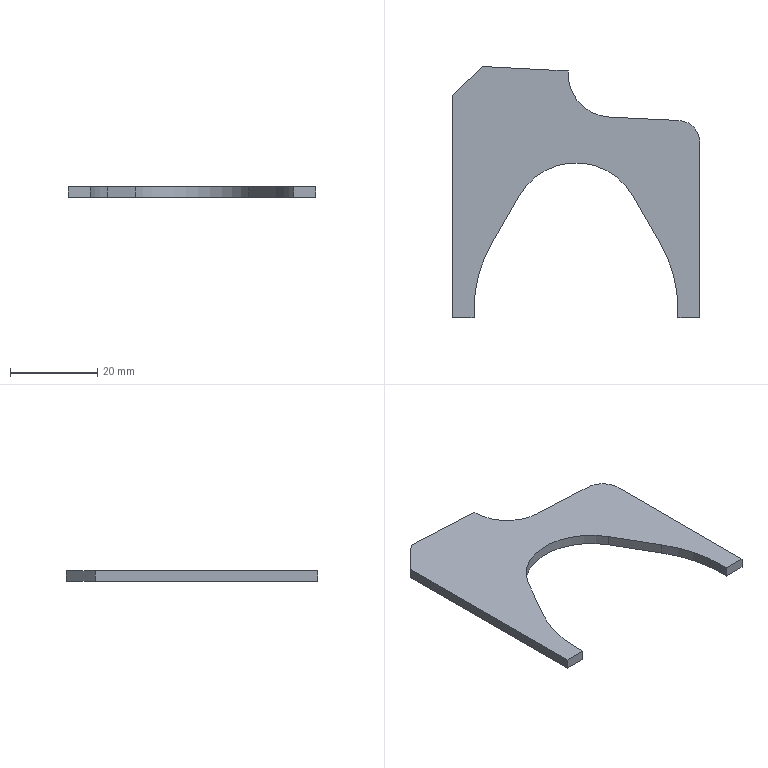Part | SolidWorks | features BreakCorner 2, FlatPattern 1, SMBaseFlange 1, SheetMetal 1 | 1 solid | 19 faces | box 56.8 x 57.632 x 2.3 mm | volume 3783 mm3 | plane 14 | cylinder 5 | commonest cylinder face diameters 60 x2 10 x1 20 x1 30 x1
STEP:
#1=CARTESIAN_POINT('',(0.,0.,0.));
#2=VERTEX_POINT('',#1);
#3=CARTESIAN_POINT('',(5.,0.,0.));
#4=VERTEX_POINT('',#3);
#5=CARTESIAN_POINT('',(5.,0.,0.));
#6=DIRECTION('',(1.,0.,0.));
#7=VECTOR('',#6,1000.);
#8=LINE('',#5,#7);
#9=EDGE_CURVE('',#2,#4,#8,.T.);
#10=ORIENTED_EDGE('',*,*,#9,.F.);
#11=CARTESIAN_POINT('',(0.,0.,-2.3));
#12=VERTEX_POINT('',#11);
#13=CARTESIAN_POINT('',(0.,0.,-2.3));
#14=DIRECTION('',(0.,0.,1.));
#15=VECTOR('',#14,1000.);
#16=LINE('',#13,#15);
#17=EDGE_CURVE('',#12,#2,#16,.T.);
#18=ORIENTED_EDGE('',*,*,#17,.F.);
#19=CARTESIAN_POINT('',(5.,0.,-2.3));
#20=VERTEX_POINT('',#19);
#21=CARTESIAN_POINT('',(5.,0.,-2.3));
#22=DIRECTION('',(1.,0.,0.));
#23=VECTOR('',#22,1000.);
#24=LINE('',#21,#23);
#25=EDGE_CURVE('',#12,#20,#24,.T.);
#26=ORIENTED_EDGE('',*,*,#25,.T.);
#27=CARTESIAN_POINT('',(5.,0.,-2.3));
#28=DIRECTION('',(0.,0.,1.));
#29=VECTOR('',#28,1000.);
#30=LINE('',#27,#29);
#31=EDGE_CURVE('',#20,#4,#30,.T.);
#32=ORIENTED_EDGE('',*,*,#31,.T.);
#33=EDGE_LOOP('',(#10,#18,#26,#32));
#34=FACE_OUTER_BOUND('',#33,.T.);
#35=CARTESIAN_POINT('',(5.,0.,-2.3));
#36=DIRECTION('',(0.,-1.,0.));
#37=DIRECTION('',(1.,0.,0.));
#38=AXIS2_PLACEMENT_3D('',#35,#36,#37);
#39=PLANE('',#38);
#40=ADVANCED_FACE('',(#34),#39,.T.);
#41=CARTESIAN_POINT('',(0.,51.,0.));
#42=VERTEX_POINT('',#41);
#43=CARTESIAN_POINT('',(0.,0.,0.));
#44=DIRECTION('',(0.,-1.,0.));
#45=VECTOR('',#44,1000.);
#46=LINE('',#43,#45);
#47=EDGE_CURVE('',#42,#2,#46,.T.);
#48=ORIENTED_EDGE('',*,*,#47,.F.);
#49=CARTESIAN_POINT('',(0.,51.,-2.3));
#50=VERTEX_POINT('',#49);
#51=CARTESIAN_POINT('',(0.,51.,-2.3));
#52=DIRECTION('',(0.,0.,-1.));
#53=VECTOR('',#52,1000.);
#54=LINE('',#51,#53);
#55=EDGE_CURVE('',#42,#50,#54,.T.);
#56=ORIENTED_EDGE('',*,*,#55,.T.);
#57=CARTESIAN_POINT('',(0.,0.,-2.3));
#58=DIRECTION('',(0.,-1.,0.));
#59=VECTOR('',#58,1000.);
#60=LINE('',#57,#59);
#61=EDGE_CURVE('',#50,#12,#60,.T.);
#62=ORIENTED_EDGE('',*,*,#61,.T.);
#63=ORIENTED_EDGE('',*,*,#17,.T.);
#64=EDGE_LOOP('',(#48,#56,#62,#63));
#65=FACE_OUTER_BOUND('',#64,.T.);
#66=CARTESIAN_POINT('',(0.,0.,-2.3));
#67=DIRECTION('',(-1.,0.,0.));
#68=DIRECTION('',(0.,0.,1.));
#69=AXIS2_PLACEMENT_3D('',#66,#67,#68);
#70=PLANE('',#69);
#71=ADVANCED_FACE('',(#65),#70,.T.);
#72=CARTESIAN_POINT('',(26.572,56.6,-2.3));
#73=VERTEX_POINT('',#72);
#74=CARTESIAN_POINT('',(6.99,57.632,-2.3));
#75=VERTEX_POINT('',#74);
#76=CARTESIAN_POINT('',(0.,58.,-2.3));
#77=DIRECTION('',(-0.9986,0.05261,0.));
#78=VECTOR('',#77,1000.);
#79=LINE('',#76,#78);
#80=EDGE_CURVE('',#73,#75,#79,.T.);
#81=ORIENTED_EDGE('',*,*,#80,.T.);
#82=CARTESIAN_POINT('',(6.99,57.632,0.));
#83=VERTEX_POINT('',#82);
#84=CARTESIAN_POINT('',(6.99,57.632,-2.3));
#85=DIRECTION('',(0.,0.,1.));
#86=VECTOR('',#85,1000.);
#87=LINE('',#84,#86);
#88=EDGE_CURVE('',#75,#83,#87,.T.);
#89=ORIENTED_EDGE('',*,*,#88,.T.);
#90=CARTESIAN_POINT('',(26.572,56.6,0.));
#91=VERTEX_POINT('',#90);
#92=CARTESIAN_POINT('',(0.,58.,0.));
#93=DIRECTION('',(-0.9986,0.05261,0.));
#94=VECTOR('',#93,1000.);
#95=LINE('',#92,#94);
#96=EDGE_CURVE('',#91,#83,#95,.T.);
#97=ORIENTED_EDGE('',*,*,#96,.F.);
#98=CARTESIAN_POINT('',(26.572,56.6,-2.3));
#99=DIRECTION('',(0.,0.,1.));
#100=VECTOR('',#99,1000.);
#101=LINE('',#98,#100);
#102=EDGE_CURVE('',#73,#91,#101,.T.);
#103=ORIENTED_EDGE('',*,*,#102,.F.);
#104=EDGE_LOOP('',(#81,#89,#97,#103));
#105=FACE_OUTER_BOUND('',#104,.T.);
#106=CARTESIAN_POINT('',(0.,58.,-2.3));
#107=DIRECTION('',(0.05261,0.9986,0.));
#108=DIRECTION('',(-0.9986,0.05261,0.));
#109=AXIS2_PLACEMENT_3D('',#106,#107,#108);
#110=PLANE('',#109);
#111=ADVANCED_FACE('',(#105),#110,.T.);
#112=CARTESIAN_POINT('',(26.572,56.,0.));
#113=VERTEX_POINT('',#112);
#114=CARTESIAN_POINT('',(26.572,56.6,0.));
#115=DIRECTION('',(0.,1.,0.));
#116=VECTOR('',#115,1000.);
#117=LINE('',#114,#116);
#118=EDGE_CURVE('',#113,#91,#117,.T.);
#119=ORIENTED_EDGE('',*,*,#118,.F.);
#120=CARTESIAN_POINT('',(26.572,56.,-2.3));
#121=VERTEX_POINT('',#120);
#122=CARTESIAN_POINT('',(26.572,56.,-2.3));
#123=DIRECTION('',(0.,0.,1.));
#124=VECTOR('',#123,1000.);
#125=LINE('',#122,#124);
#126=EDGE_CURVE('',#121,#113,#125,.T.);
#127=ORIENTED_EDGE('',*,*,#126,.F.);
#128=CARTESIAN_POINT('',(26.572,56.6,-2.3));
#129=DIRECTION('',(0.,1.,0.));
#130=VECTOR('',#129,1000.);
#131=LINE('',#128,#130);
#132=EDGE_CURVE('',#121,#73,#131,.T.);
#133=ORIENTED_EDGE('',*,*,#132,.T.);
#134=ORIENTED_EDGE('',*,*,#102,.T.);
#135=EDGE_LOOP('',(#119,#127,#133,#134));
#136=FACE_OUTER_BOUND('',#135,.T.);
#137=CARTESIAN_POINT('',(26.572,56.6,-2.3));
#138=DIRECTION('',(1.,0.,0.));
#139=DIRECTION('',(0.,1.,0.));
#140=AXIS2_PLACEMENT_3D('',#137,#138,#139);
#141=PLANE('',#140);
#142=ADVANCED_FACE('',(#136),#141,.T.);
#143=CARTESIAN_POINT('',(36.085,46.012,0.));
#144=VERTEX_POINT('',#143);
#145=CARTESIAN_POINT('',(36.572,56.,0.));
#146=DIRECTION('',(0.,0.,-1.));
#147=DIRECTION('',(-1.,0.,0.));
#148=AXIS2_PLACEMENT_3D('',#145,#146,#147);
#149=CIRCLE('',#148,10.);
#150=EDGE_CURVE('',#144,#113,#149,.T.);
#151=ORIENTED_EDGE('',*,*,#150,.F.);
#152=CARTESIAN_POINT('',(36.085,46.012,-2.3));
#153=VERTEX_POINT('',#152);
#154=CARTESIAN_POINT('',(36.085,46.012,-2.3));
#155=DIRECTION('',(0.,0.,1.));
#156=VECTOR('',#155,1000.);
#157=LINE('',#154,#156);
#158=EDGE_CURVE('',#153,#144,#157,.T.);
#159=ORIENTED_EDGE('',*,*,#158,.F.);
#160=CARTESIAN_POINT('',(36.572,56.,-2.3));
#161=DIRECTION('',(0.,0.,-1.));
#162=DIRECTION('',(-1.,0.,0.));
#163=AXIS2_PLACEMENT_3D('',#160,#161,#162);
#164=CIRCLE('',#163,10.);
#165=EDGE_CURVE('',#153,#121,#164,.T.);
#166=ORIENTED_EDGE('',*,*,#165,.T.);
#167=ORIENTED_EDGE('',*,*,#126,.T.);
#168=EDGE_LOOP('',(#151,#159,#166,#167));
#169=FACE_OUTER_BOUND('',#168,.T.);
#170=CARTESIAN_POINT('',(36.572,56.,-2.3));
#171=DIRECTION('',(0.,0.,1.));
#172=DIRECTION('',(1.,0.,0.));
#173=AXIS2_PLACEMENT_3D('',#170,#171,#172);
#174=CYLINDRICAL_SURFACE('',#173,10.);
#175=ADVANCED_FACE('',(#169),#174,.F.);
#176=CARTESIAN_POINT('',(52.044,45.232,0.));
#177=VERTEX_POINT('',#176);
#178=CARTESIAN_POINT('',(36.085,46.012,0.));
#179=DIRECTION('',(-0.9988,0.04879,0.));
#180=VECTOR('',#179,1000.);
#181=LINE('',#178,#180);
#182=EDGE_CURVE('',#177,#144,#181,.T.);
#183=ORIENTED_EDGE('',*,*,#182,.F.);
#184=CARTESIAN_POINT('',(52.044,45.232,-2.3));
#185=VERTEX_POINT('',#184);
#186=CARTESIAN_POINT('',(52.044,45.232,-2.3));
#187=DIRECTION('',(0.,0.,-1.));
#188=VECTOR('',#187,1000.);
#189=LINE('',#186,#188);
#190=EDGE_CURVE('',#177,#185,#189,.T.);
#191=ORIENTED_EDGE('',*,*,#190,.T.);
#192=CARTESIAN_POINT('',(36.085,46.012,-2.3));
#193=DIRECTION('',(-0.9988,0.04879,0.));
#194=VECTOR('',#193,1000.);
#195=LINE('',#192,#194);
#196=EDGE_CURVE('',#185,#153,#195,.T.);
#197=ORIENTED_EDGE('',*,*,#196,.T.);
#198=ORIENTED_EDGE('',*,*,#158,.T.);
#199=EDGE_LOOP('',(#183,#191,#197,#198));
#200=FACE_OUTER_BOUND('',#199,.T.);
#201=CARTESIAN_POINT('',(36.085,46.012,-2.3));
#202=DIRECTION('',(0.04879,0.9988,0.));
#203=DIRECTION('',(-0.9988,0.04879,0.));
#204=AXIS2_PLACEMENT_3D('',#201,#202,#203);
#205=PLANE('',#204);
#206=ADVANCED_FACE('',(#200),#205,.T.);
#207=CARTESIAN_POINT('',(56.8,0.,-2.3));
#208=VERTEX_POINT('',#207);
#209=CARTESIAN_POINT('',(56.8,40.238,-2.3));
#210=VERTEX_POINT('',#209);
#211=CARTESIAN_POINT('',(56.8,45.,-2.3));
#212=DIRECTION('',(0.,1.,0.));
#213=VECTOR('',#212,1000.);
#214=LINE('',#211,#213);
#215=EDGE_CURVE('',#208,#210,#214,.T.);
#216=ORIENTED_EDGE('',*,*,#215,.T.);
#217=CARTESIAN_POINT('',(56.8,40.238,0.));
#218=VERTEX_POINT('',#217);
#219=CARTESIAN_POINT('',(56.8,40.238,-2.3));
#220=DIRECTION('',(0.,0.,1.));
#221=VECTOR('',#220,1000.);
#222=LINE('',#219,#221);
#223=EDGE_CURVE('',#210,#218,#222,.T.);
#224=ORIENTED_EDGE('',*,*,#223,.T.);
#225=CARTESIAN_POINT('',(56.8,0.,0.));
#226=VERTEX_POINT('',#225);
#227=CARTESIAN_POINT('',(56.8,45.,0.));
#228=DIRECTION('',(0.,1.,0.));
#229=VECTOR('',#228,1000.);
#230=LINE('',#227,#229);
#231=EDGE_CURVE('',#226,#218,#230,.T.);
#232=ORIENTED_EDGE('',*,*,#231,.F.);
#233=CARTESIAN_POINT('',(56.8,0.,-2.3));
#234=DIRECTION('',(0.,0.,1.));
#235=VECTOR('',#234,1000.);
#236=LINE('',#233,#235);
#237=EDGE_CURVE('',#208,#226,#236,.T.);
#238=ORIENTED_EDGE('',*,*,#237,.F.);
#239=EDGE_LOOP('',(#216,#224,#232,#238));
#240=FACE_OUTER_BOUND('',#239,.T.);
#241=CARTESIAN_POINT('',(56.8,45.,-2.3));
#242=DIRECTION('',(1.,0.,0.));
#243=DIRECTION('',(0.,1.,0.));
#244=AXIS2_PLACEMENT_3D('',#241,#242,#243);
#245=PLANE('',#244);
#246=ADVANCED_FACE('',(#240),#245,.T.);
#247=CARTESIAN_POINT('',(51.8,0.,0.));
#248=VERTEX_POINT('',#247);
#249=CARTESIAN_POINT('',(56.8,0.,0.));
#250=DIRECTION('',(1.,0.,0.));
#251=VECTOR('',#250,1000.);
#252=LINE('',#249,#251);
#253=EDGE_CURVE('',#248,#226,#252,.T.);
#254=ORIENTED_EDGE('',*,*,#253,.F.);
#255=CARTESIAN_POINT('',(51.8,0.,-2.3));
#256=VERTEX_POINT('',#255);
#257=CARTESIAN_POINT('',(51.8,0.,-2.3));
#258=DIRECTION('',(0.,0.,1.));
#259=VECTOR('',#258,1000.);
#260=LINE('',#257,#259);
#261=EDGE_CURVE('',#256,#248,#260,.T.);
#262=ORIENTED_EDGE('',*,*,#261,.F.);
#263=CARTESIAN_POINT('',(56.8,0.,-2.3));
#264=DIRECTION('',(1.,0.,0.));
#265=VECTOR('',#264,1000.);
#266=LINE('',#263,#265);
#267=EDGE_CURVE('',#256,#208,#266,.T.);
#268=ORIENTED_EDGE('',*,*,#267,.T.);
#269=ORIENTED_EDGE('',*,*,#237,.T.);
#270=EDGE_LOOP('',(#254,#262,#268,#269));
#271=FACE_OUTER_BOUND('',#270,.T.);
#272=CARTESIAN_POINT('',(56.8,0.,-2.3));
#273=DIRECTION('',(0.,-1.,0.));
#274=DIRECTION('',(1.,0.,0.));
#275=AXIS2_PLACEMENT_3D('',#272,#273,#274);
#276=PLANE('',#275);
#277=ADVANCED_FACE('',(#271),#276,.T.);
#278=CARTESIAN_POINT('',(51.8,1.95,0.));
#279=VERTEX_POINT('',#278);
#280=CARTESIAN_POINT('',(51.8,0.,0.));
#281=DIRECTION('',(0.,-1.,0.));
#282=VECTOR('',#281,1000.);
#283=LINE('',#280,#282);
#284=EDGE_CURVE('',#279,#248,#283,.T.);
#285=ORIENTED_EDGE('',*,*,#284,.F.);
#286=CARTESIAN_POINT('',(51.8,1.95,-2.3));
#287=VERTEX_POINT('',#286);
#288=CARTESIAN_POINT('',(51.8,1.95,-2.3));
#289=DIRECTION('',(0.,0.,1.));
#290=VECTOR('',#289,1000.);
#291=LINE('',#288,#290);
#292=EDGE_CURVE('',#287,#279,#291,.T.);
#293=ORIENTED_EDGE('',*,*,#292,.F.);
#294=CARTESIAN_POINT('',(51.8,0.,-2.3));
#295=DIRECTION('',(0.,-1.,0.));
#296=VECTOR('',#295,1000.);
#297=LINE('',#294,#296);
#298=EDGE_CURVE('',#287,#256,#297,.T.);
#299=ORIENTED_EDGE('',*,*,#298,.T.);
#300=ORIENTED_EDGE('',*,*,#261,.T.);
#301=EDGE_LOOP('',(#285,#293,#299,#300));
#302=FACE_OUTER_BOUND('',#301,.T.);
#303=CARTESIAN_POINT('',(51.8,0.,-2.3));
#304=DIRECTION('',(-1.,0.,0.));
#305=DIRECTION('',(0.,0.,1.));
#306=AXIS2_PLACEMENT_3D('',#303,#304,#305);
#307=PLANE('',#306);
#308=ADVANCED_FACE('',(#302),#307,.T.);
#309=CARTESIAN_POINT('',(47.77,16.969,0.));
#310=VERTEX_POINT('',#309);
#311=CARTESIAN_POINT('',(21.8,1.95,0.));
#312=DIRECTION('',(0.,0.,-1.));
#313=DIRECTION('',(1.,0.,0.));
#314=AXIS2_PLACEMENT_3D('',#311,#312,#313);
#315=CIRCLE('',#314,30.);
#316=EDGE_CURVE('',#310,#279,#315,.T.);
#317=ORIENTED_EDGE('',*,*,#316,.F.);
#318=CARTESIAN_POINT('',(47.77,16.969,-2.3));
#319=VERTEX_POINT('',#318);
#320=CARTESIAN_POINT('',(47.77,16.969,-2.3));
#321=DIRECTION('',(0.,0.,1.));
#322=VECTOR('',#321,1000.);
#323=LINE('',#320,#322);
#324=EDGE_CURVE('',#319,#310,#323,.T.);
#325=ORIENTED_EDGE('',*,*,#324,.F.);
#326=CARTESIAN_POINT('',(21.8,1.95,-2.3));
#327=DIRECTION('',(0.,0.,-1.));
#328=DIRECTION('',(1.,0.,0.));
#329=AXIS2_PLACEMENT_3D('',#326,#327,#328);
#330=CIRCLE('',#329,30.);
#331=EDGE_CURVE('',#319,#287,#330,.T.);
#332=ORIENTED_EDGE('',*,*,#331,.T.);
#333=ORIENTED_EDGE('',*,*,#292,.T.);
#334=EDGE_LOOP('',(#317,#325,#332,#333));
#335=FACE_OUTER_BOUND('',#334,.T.);
#336=CARTESIAN_POINT('',(21.8,1.95,-2.3));
#337=DIRECTION('',(0.,0.,1.));
#338=DIRECTION('',(1.,0.,0.));
#339=AXIS2_PLACEMENT_3D('',#336,#337,#338);
#340=CYLINDRICAL_SURFACE('',#339,30.);
#341=ADVANCED_FACE('',(#335),#340,.F.);
#342=CARTESIAN_POINT('',(41.385,28.009,0.));
#343=VERTEX_POINT('',#342);
#344=CARTESIAN_POINT('',(47.77,16.969,0.));
#345=DIRECTION('',(0.5006,-0.8657,0.));
#346=VECTOR('',#345,1000.);
#347=LINE('',#344,#346);
#348=EDGE_CURVE('',#343,#310,#347,.T.);
#349=ORIENTED_EDGE('',*,*,#348,.F.);
#350=CARTESIAN_POINT('',(41.385,28.009,-2.3));
#351=VERTEX_POINT('',#350);
#352=CARTESIAN_POINT('',(41.385,28.009,-2.3));
#353=DIRECTION('',(0.,0.,1.));
#354=VECTOR('',#353,1000.);
#355=LINE('',#352,#354);
#356=EDGE_CURVE('',#351,#343,#355,.T.);
#357=ORIENTED_EDGE('',*,*,#356,.F.);
#358=CARTESIAN_POINT('',(47.77,16.969,-2.3));
#359=DIRECTION('',(0.5006,-0.8657,0.));
#360=VECTOR('',#359,1000.);
#361=LINE('',#358,#360);
#362=EDGE_CURVE('',#351,#319,#361,.T.);
#363=ORIENTED_EDGE('',*,*,#362,.T.);
#364=ORIENTED_EDGE('',*,*,#324,.T.);
#365=EDGE_LOOP('',(#349,#357,#363,#364));
#366=FACE_OUTER_BOUND('',#365,.T.);
#367=CARTESIAN_POINT('',(47.77,16.969,-2.3));
#368=DIRECTION('',(-0.8657,-0.5006,0.));
#369=DIRECTION('',(0.5006,-0.8657,0.));
#370=AXIS2_PLACEMENT_3D('',#367,#368,#369);
#371=PLANE('',#370);
#372=ADVANCED_FACE('',(#366),#371,.T.);
#373=CARTESIAN_POINT('',(15.415,28.009,0.));
#374=VERTEX_POINT('',#373);
#375=CARTESIAN_POINT('',(28.4,20.5,0.));
#376=DIRECTION('',(0.,0.,-1.));
#377=DIRECTION('',(1.,0.,0.));
#378=AXIS2_PLACEMENT_3D('',#375,#376,#377);
#379=CIRCLE('',#378,15.);
#380=EDGE_CURVE('',#374,#343,#379,.T.);
#381=ORIENTED_EDGE('',*,*,#380,.F.);
#382=CARTESIAN_POINT('',(15.415,28.009,-2.3));
#383=VERTEX_POINT('',#382);
#384=CARTESIAN_POINT('',(15.415,28.009,-2.3));
#385=DIRECTION('',(0.,0.,1.));
#386=VECTOR('',#385,1000.);
#387=LINE('',#384,#386);
#388=EDGE_CURVE('',#383,#374,#387,.T.);
#389=ORIENTED_EDGE('',*,*,#388,.F.);
#390=CARTESIAN_POINT('',(28.4,20.5,-2.3));
#391=DIRECTION('',(0.,0.,-1.));
#392=DIRECTION('',(1.,0.,0.));
#393=AXIS2_PLACEMENT_3D('',#390,#391,#392);
#394=CIRCLE('',#393,15.);
#395=EDGE_CURVE('',#383,#351,#394,.T.);
#396=ORIENTED_EDGE('',*,*,#395,.T.);
#397=ORIENTED_EDGE('',*,*,#356,.T.);
#398=EDGE_LOOP('',(#381,#389,#396,#397));
#399=FACE_OUTER_BOUND('',#398,.T.);
#400=CARTESIAN_POINT('',(28.4,20.5,-2.3));
#401=DIRECTION('',(0.,0.,1.));
#402=DIRECTION('',(1.,0.,0.));
#403=AXIS2_PLACEMENT_3D('',#400,#401,#402);
#404=CYLINDRICAL_SURFACE('',#403,15.);
#405=ADVANCED_FACE('',(#399),#404,.F.);
#406=CARTESIAN_POINT('',(9.03,16.969,0.));
#407=VERTEX_POINT('',#406);
#408=CARTESIAN_POINT('',(15.415,28.009,0.));
#409=DIRECTION('',(0.5006,0.8657,0.));
#410=VECTOR('',#409,1000.);
#411=LINE('',#408,#410);
#412=EDGE_CURVE('',#407,#374,#411,.T.);
#413=ORIENTED_EDGE('',*,*,#412,.F.);
#414=CARTESIAN_POINT('',(9.03,16.969,-2.3));
#415=VERTEX_POINT('',#414);
#416=CARTESIAN_POINT('',(9.03,16.969,-2.3));
#417=DIRECTION('',(0.,0.,1.));
#418=VECTOR('',#417,1000.);
#419=LINE('',#416,#418);
#420=EDGE_CURVE('',#415,#407,#419,.T.);
#421=ORIENTED_EDGE('',*,*,#420,.F.);
#422=CARTESIAN_POINT('',(15.415,28.009,-2.3));
#423=DIRECTION('',(0.5006,0.8657,0.));
#424=VECTOR('',#423,1000.);
#425=LINE('',#422,#424);
#426=EDGE_CURVE('',#415,#383,#425,.T.);
#427=ORIENTED_EDGE('',*,*,#426,.T.);
#428=ORIENTED_EDGE('',*,*,#388,.T.);
#429=EDGE_LOOP('',(#413,#421,#427,#428));
#430=FACE_OUTER_BOUND('',#429,.T.);
#431=CARTESIAN_POINT('',(15.415,28.009,-2.3));
#432=DIRECTION('',(0.8657,-0.5006,0.));
#433=DIRECTION('',(0.5006,0.8657,0.));
#434=AXIS2_PLACEMENT_3D('',#431,#432,#433);
#435=PLANE('',#434);
#436=ADVANCED_FACE('',(#430),#435,.T.);
#437=CARTESIAN_POINT('',(5.,1.95,0.));
#438=VERTEX_POINT('',#437);
#439=CARTESIAN_POINT('',(35.,1.95,0.));
#440=DIRECTION('',(0.,0.,-1.));
#441=DIRECTION('',(-1.,0.,0.));
#442=AXIS2_PLACEMENT_3D('',#439,#440,#441);
#443=CIRCLE('',#442,30.);
#444=EDGE_CURVE('',#438,#407,#443,.T.);
#445=ORIENTED_EDGE('',*,*,#444,.F.);
#446=CARTESIAN_POINT('',(5.,1.95,-2.3));
#447=VERTEX_POINT('',#446);
#448=CARTESIAN_POINT('',(5.,1.95,-2.3));
#449=DIRECTION('',(0.,0.,1.));
#450=VECTOR('',#449,1000.);
#451=LINE('',#448,#450);
#452=EDGE_CURVE('',#447,#438,#451,.T.);
#453=ORIENTED_EDGE('',*,*,#452,.F.);
#454=CARTESIAN_POINT('',(35.,1.95,-2.3));
#455=DIRECTION('',(0.,0.,-1.));
#456=DIRECTION('',(-1.,0.,0.));
#457=AXIS2_PLACEMENT_3D('',#454,#455,#456);
#458=CIRCLE('',#457,30.);
#459=EDGE_CURVE('',#447,#415,#458,.T.);
#460=ORIENTED_EDGE('',*,*,#459,.T.);
#461=ORIENTED_EDGE('',*,*,#420,.T.);
#462=EDGE_LOOP('',(#445,#453,#460,#461));
#463=FACE_OUTER_BOUND('',#462,.T.);
#464=CARTESIAN_POINT('',(35.,1.95,-2.3));
#465=DIRECTION('',(0.,0.,1.));
#466=DIRECTION('',(1.,0.,0.));
#467=AXIS2_PLACEMENT_3D('',#464,#465,#466);
#468=CYLINDRICAL_SURFACE('',#467,30.);
#469=ADVANCED_FACE('',(#463),#468,.F.);
#470=CARTESIAN_POINT('',(5.,1.95,0.));
#471=DIRECTION('',(0.,1.,0.));
#472=VECTOR('',#471,1000.);
#473=LINE('',#470,#472);
#474=EDGE_CURVE('',#4,#438,#473,.T.);
#475=ORIENTED_EDGE('',*,*,#474,.F.);
#476=ORIENTED_EDGE('',*,*,#31,.F.);
#477=CARTESIAN_POINT('',(5.,1.95,-2.3));
#478=DIRECTION('',(0.,1.,0.));
#479=VECTOR('',#478,1000.);
#480=LINE('',#477,#479);
#481=EDGE_CURVE('',#20,#447,#480,.T.);
#482=ORIENTED_EDGE('',*,*,#481,.T.);
#483=ORIENTED_EDGE('',*,*,#452,.T.);
#484=EDGE_LOOP('',(#475,#476,#482,#483));
#485=FACE_OUTER_BOUND('',#484,.T.);
#486=CARTESIAN_POINT('',(5.,1.95,-2.3));
#487=DIRECTION('',(1.,0.,0.));
#488=DIRECTION('',(0.,1.,0.));
#489=AXIS2_PLACEMENT_3D('',#486,#487,#488);
#490=PLANE('',#489);
#491=ADVANCED_FACE('',(#485),#490,.T.);
#492=ORIENTED_EDGE('',*,*,#196,.F.);
#493=CARTESIAN_POINT('',(51.8,40.238,-2.3));
#494=DIRECTION('',(0.,0.,-1.));
#495=DIRECTION('',(-1.,0.,0.));
#496=AXIS2_PLACEMENT_3D('',#493,#494,#495);
#497=CIRCLE('',#496,5.);
#498=EDGE_CURVE('',#185,#210,#497,.T.);
#499=ORIENTED_EDGE('',*,*,#498,.T.);
#500=ORIENTED_EDGE('',*,*,#215,.F.);
#501=ORIENTED_EDGE('',*,*,#267,.F.);
#502=ORIENTED_EDGE('',*,*,#298,.F.);
#503=ORIENTED_EDGE('',*,*,#331,.F.);
#504=ORIENTED_EDGE('',*,*,#362,.F.);
#505=ORIENTED_EDGE('',*,*,#395,.F.);
#506=ORIENTED_EDGE('',*,*,#426,.F.);
#507=ORIENTED_EDGE('',*,*,#459,.F.);
#508=ORIENTED_EDGE('',*,*,#481,.F.);
#509=ORIENTED_EDGE('',*,*,#25,.F.);
#510=ORIENTED_EDGE('',*,*,#61,.F.);
#511=CARTESIAN_POINT('',(21.745,71.629,-2.3));
#512=DIRECTION('',(0.7255,0.6883,0.));
#513=VECTOR('',#512,1000.);
#514=LINE('',#511,#513);
#515=EDGE_CURVE('',#50,#75,#514,.T.);
#516=ORIENTED_EDGE('',*,*,#515,.T.);
#517=ORIENTED_EDGE('',*,*,#80,.F.);
#518=ORIENTED_EDGE('',*,*,#132,.F.);
#519=ORIENTED_EDGE('',*,*,#165,.F.);
#520=EDGE_LOOP('',(#492,#499,#500,#501,#502,#503,#504,#505,#506,#507,#508,#509,#510,#516,#517,#518,#519));
#521=FACE_OUTER_BOUND('',#520,.T.);
#522=CARTESIAN_POINT('',(36.572,56.,-2.3));
#523=DIRECTION('',(0.,0.,-1.));
#524=DIRECTION('',(-1.,0.,0.));
#525=AXIS2_PLACEMENT_3D('',#522,#523,#524);
#526=PLANE('',#525);
#527=ADVANCED_FACE('',(#521),#526,.T.);
#528=ORIENTED_EDGE('',*,*,#231,.T.);
#529=CARTESIAN_POINT('',(51.8,40.238,0.));
#530=DIRECTION('',(0.,0.,1.));
#531=DIRECTION('',(-1.,0.,0.));
#532=AXIS2_PLACEMENT_3D('',#529,#530,#531);
#533=CIRCLE('',#532,5.);
#534=EDGE_CURVE('',#218,#177,#533,.T.);
#535=ORIENTED_EDGE('',*,*,#534,.T.);
#536=ORIENTED_EDGE('',*,*,#182,.T.);
#537=ORIENTED_EDGE('',*,*,#150,.T.);
#538=ORIENTED_EDGE('',*,*,#118,.T.);
#539=ORIENTED_EDGE('',*,*,#96,.T.);
#540=CARTESIAN_POINT('',(6.99,57.632,0.));
#541=DIRECTION('',(-0.7255,-0.6883,0.));
#542=VECTOR('',#541,1000.);
#543=LINE('',#540,#542);
#544=EDGE_CURVE('',#83,#42,#543,.T.);
#545=ORIENTED_EDGE('',*,*,#544,.T.);
#546=ORIENTED_EDGE('',*,*,#47,.T.);
#547=ORIENTED_EDGE('',*,*,#9,.T.);
#548=ORIENTED_EDGE('',*,*,#474,.T.);
#549=ORIENTED_EDGE('',*,*,#444,.T.);
#550=ORIENTED_EDGE('',*,*,#412,.T.);
#551=ORIENTED_EDGE('',*,*,#380,.T.);
#552=ORIENTED_EDGE('',*,*,#348,.T.);
#553=ORIENTED_EDGE('',*,*,#316,.T.);
#554=ORIENTED_EDGE('',*,*,#284,.T.);
#555=ORIENTED_EDGE('',*,*,#253,.T.);
#556=EDGE_LOOP('',(#528,#535,#536,#537,#538,#539,#545,#546,#547,#548,#549,#550,#551,#552,#553,#554,#555));
#557=FACE_OUTER_BOUND('',#556,.T.);
#558=CARTESIAN_POINT('',(36.572,56.,0.));
#559=DIRECTION('',(0.,0.,-1.));
#560=DIRECTION('',(-1.,0.,0.));
#561=AXIS2_PLACEMENT_3D('',#558,#559,#560);
#562=PLANE('',#561);
#563=ADVANCED_FACE('',(#557),#562,.F.);
#564=ORIENTED_EDGE('',*,*,#515,.F.);
#565=ORIENTED_EDGE('',*,*,#55,.F.);
#566=ORIENTED_EDGE('',*,*,#544,.F.);
#567=ORIENTED_EDGE('',*,*,#88,.F.);
#568=EDGE_LOOP('',(#564,#565,#566,#567));
#569=FACE_OUTER_BOUND('',#568,.T.);
#570=CARTESIAN_POINT('',(6.99,57.632,-2.3));
#571=DIRECTION('',(0.6883,-0.7255,0.));
#572=DIRECTION('',(0.,0.,1.));
#573=AXIS2_PLACEMENT_3D('',#570,#571,#572);
#574=PLANE('',#573);
#575=ADVANCED_FACE('',(#569),#574,.F.);
#576=ORIENTED_EDGE('',*,*,#498,.F.);
#577=ORIENTED_EDGE('',*,*,#190,.F.);
#578=ORIENTED_EDGE('',*,*,#534,.F.);
#579=ORIENTED_EDGE('',*,*,#223,.F.);
#580=EDGE_LOOP('',(#576,#577,#578,#579));
#581=FACE_OUTER_BOUND('',#580,.T.);
#582=CARTESIAN_POINT('',(51.8,40.238,-2.3));
#583=DIRECTION('',(0.,0.,1.));
#584=DIRECTION('',(1.,0.,0.));
#585=AXIS2_PLACEMENT_3D('',#582,#583,#584);
#586=CYLINDRICAL_SURFACE('',#585,5.);
#587=ADVANCED_FACE('',(#581),#586,.T.);
#588=CLOSED_SHELL('',(#40,#71,#111,#142,#175,#206,#246,#277,#308,#341,#372,#405,#436,#469,#491,#527,#563,#575,#587));
#589=MANIFOLD_SOLID_BREP('',#588);
#590=CARTESIAN_POINT('',(0.,0.,0.));
#591=DIRECTION('',(0.,0.,1.));
#592=DIRECTION('',(1.,0.,0.));
#593=AXIS2_PLACEMENT_3D('',#590,#591,#592);
#594=(LENGTH_UNIT()NAMED_UNIT(*)SI_UNIT(.MILLI.,.METRE.));
#595=UNCERTAINTY_MEASURE_WITH_UNIT(LENGTH_MEASURE(0.00001),#594,'','');
#596=(NAMED_UNIT(*)PLANE_ANGLE_UNIT()SI_UNIT($,.RADIAN.));
#597=(NAMED_UNIT(*)SI_UNIT($,.STERADIAN.)SOLID_ANGLE_UNIT());
#598=(GEOMETRIC_REPRESENTATION_CONTEXT(3)GLOBAL_UNCERTAINTY_ASSIGNED_CONTEXT((#595))GLOBAL_UNIT_ASSIGNED_CONTEXT((#594,#596,#597))REPRESENTATION_CONTEXT('',''));
#599=ADVANCED_BREP_SHAPE_REPRESENTATION('',(#589,#593),#598);